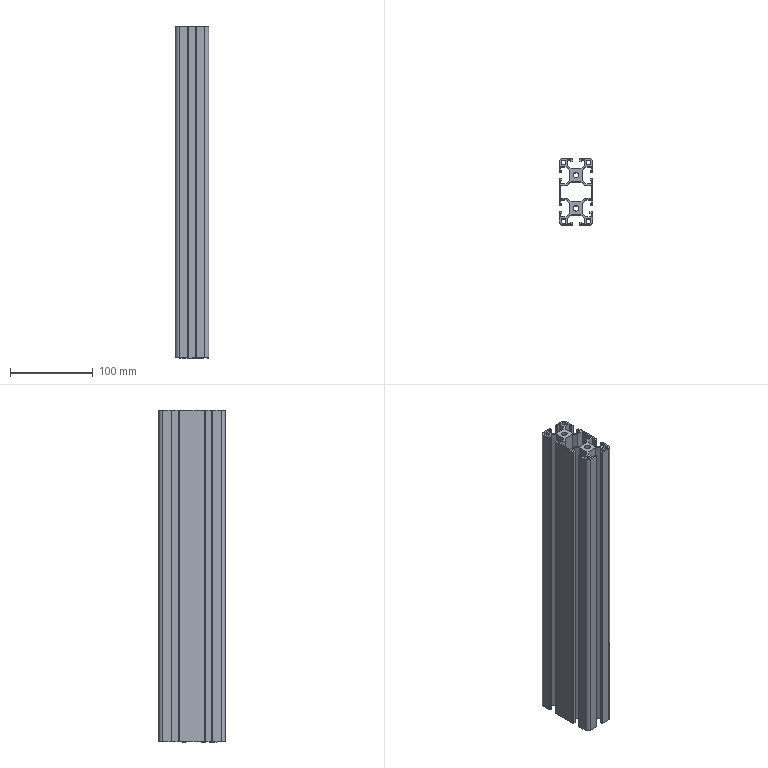Part | SolidWorks | features BaseBody 1 | 1 solid | 155 faces | box 40.002 x 80 x 400 mm | volume 393757 mm3 | plane 142 | cylinder 13 | commonest cylinder face diameters 9 x5 5 x4 6.8 x4